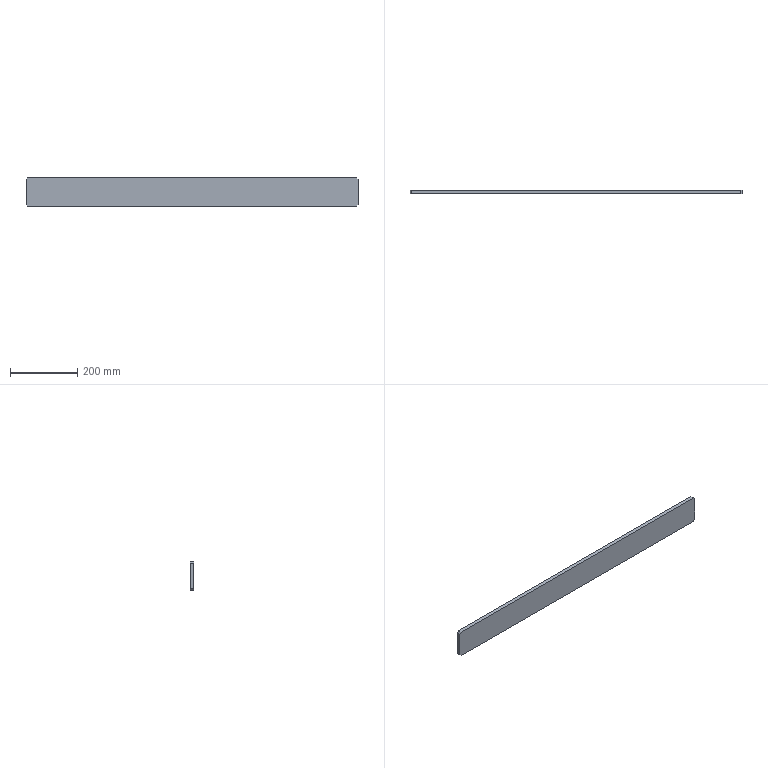Part | STEP file | Guide wheel mechanism revised.sldasm-Part-67 | 1 solid | 10 faces | box 985 x 10 x 85 mm | volume 836750 mm3 | plane 10
STEP:
#1=CARTESIAN_POINT('',(-492.5,265.,-37.5));
#2=VERTEX_POINT('',#1);
#3=CARTESIAN_POINT('',(-492.5,265.,37.5));
#4=VERTEX_POINT('',#3);
#5=CARTESIAN_POINT('',(-492.5,265.,-42.5));
#6=DIRECTION('',(0.,0.,1.));
#7=VECTOR('',#6,1000.);
#8=LINE('',#5,#7);
#9=EDGE_CURVE('',#2,#4,#8,.T.);
#10=ORIENTED_EDGE('',*,*,#9,.F.);
#11=CARTESIAN_POINT('',(-492.5,255.,-37.5));
#12=VERTEX_POINT('',#11);
#13=CARTESIAN_POINT('',(-492.5,265.,-37.5));
#14=DIRECTION('',(0.,-1.,0.));
#15=VECTOR('',#14,1000.);
#16=LINE('',#13,#15);
#17=EDGE_CURVE('',#2,#12,#16,.T.);
#18=ORIENTED_EDGE('',*,*,#17,.T.);
#19=CARTESIAN_POINT('',(-492.5,255.,37.5));
#20=VERTEX_POINT('',#19);
#21=CARTESIAN_POINT('',(-492.5,255.,-42.5));
#22=DIRECTION('',(0.,0.,1.));
#23=VECTOR('',#22,1000.);
#24=LINE('',#21,#23);
#25=EDGE_CURVE('',#12,#20,#24,.T.);
#26=ORIENTED_EDGE('',*,*,#25,.T.);
#27=CARTESIAN_POINT('',(-492.5,265.,37.5));
#28=DIRECTION('',(0.,1.,0.));
#29=VECTOR('',#28,1000.);
#30=LINE('',#27,#29);
#31=EDGE_CURVE('',#20,#4,#30,.T.);
#32=ORIENTED_EDGE('',*,*,#31,.T.);
#33=EDGE_LOOP('',(#10,#18,#26,#32));
#34=FACE_OUTER_BOUND('',#33,.T.);
#35=CARTESIAN_POINT('',(-492.5,265.,-42.5));
#36=DIRECTION('',(1.,0.,0.));
#37=DIRECTION('',(0.,0.,-1.));
#38=AXIS2_PLACEMENT_3D('',#35,#36,#37);
#39=PLANE('',#38);
#40=ADVANCED_FACE('',(#34),#39,.F.);
#41=CARTESIAN_POINT('',(-487.5,255.,42.5));
#42=VERTEX_POINT('',#41);
#43=CARTESIAN_POINT('',(487.5,255.,42.5));
#44=VERTEX_POINT('',#43);
#45=CARTESIAN_POINT('',(-492.5,255.,42.5));
#46=DIRECTION('',(1.,0.,0.));
#47=VECTOR('',#46,1000.);
#48=LINE('',#45,#47);
#49=EDGE_CURVE('',#42,#44,#48,.T.);
#50=ORIENTED_EDGE('',*,*,#49,.T.);
#51=CARTESIAN_POINT('',(487.5,265.,42.5));
#52=VERTEX_POINT('',#51);
#53=CARTESIAN_POINT('',(487.5,265.,42.5));
#54=DIRECTION('',(0.,1.,0.));
#55=VECTOR('',#54,1000.);
#56=LINE('',#53,#55);
#57=EDGE_CURVE('',#44,#52,#56,.T.);
#58=ORIENTED_EDGE('',*,*,#57,.T.);
#59=CARTESIAN_POINT('',(-487.5,265.,42.5));
#60=VERTEX_POINT('',#59);
#61=CARTESIAN_POINT('',(-492.5,265.,42.5));
#62=DIRECTION('',(1.,0.,0.));
#63=VECTOR('',#62,1000.);
#64=LINE('',#61,#63);
#65=EDGE_CURVE('',#60,#52,#64,.T.);
#66=ORIENTED_EDGE('',*,*,#65,.F.);
#67=CARTESIAN_POINT('',(-487.5,265.,42.5));
#68=DIRECTION('',(0.,-1.,0.));
#69=VECTOR('',#68,1000.);
#70=LINE('',#67,#69);
#71=EDGE_CURVE('',#60,#42,#70,.T.);
#72=ORIENTED_EDGE('',*,*,#71,.T.);
#73=EDGE_LOOP('',(#50,#58,#66,#72));
#74=FACE_OUTER_BOUND('',#73,.T.);
#75=CARTESIAN_POINT('',(-492.5,265.,42.5));
#76=DIRECTION('',(0.,0.,-1.));
#77=DIRECTION('',(-1.,0.,0.));
#78=AXIS2_PLACEMENT_3D('',#75,#76,#77);
#79=PLANE('',#78);
#80=ADVANCED_FACE('',(#74),#79,.F.);
#81=CARTESIAN_POINT('',(492.5,255.,37.5));
#82=VERTEX_POINT('',#81);
#83=CARTESIAN_POINT('',(492.5,255.,-37.5));
#84=VERTEX_POINT('',#83);
#85=CARTESIAN_POINT('',(492.5,255.,-42.5));
#86=DIRECTION('',(0.,0.,-1.));
#87=VECTOR('',#86,1000.);
#88=LINE('',#85,#87);
#89=EDGE_CURVE('',#82,#84,#88,.T.);
#90=ORIENTED_EDGE('',*,*,#89,.T.);
#91=CARTESIAN_POINT('',(492.5,265.,-37.5));
#92=VERTEX_POINT('',#91);
#93=CARTESIAN_POINT('',(492.5,265.,-37.5));
#94=DIRECTION('',(0.,1.,0.));
#95=VECTOR('',#94,1000.);
#96=LINE('',#93,#95);
#97=EDGE_CURVE('',#84,#92,#96,.T.);
#98=ORIENTED_EDGE('',*,*,#97,.T.);
#99=CARTESIAN_POINT('',(492.5,265.,37.5));
#100=VERTEX_POINT('',#99);
#101=CARTESIAN_POINT('',(492.5,265.,-42.5));
#102=DIRECTION('',(0.,0.,-1.));
#103=VECTOR('',#102,1000.);
#104=LINE('',#101,#103);
#105=EDGE_CURVE('',#100,#92,#104,.T.);
#106=ORIENTED_EDGE('',*,*,#105,.F.);
#107=CARTESIAN_POINT('',(492.5,265.,37.5));
#108=DIRECTION('',(0.,-1.,0.));
#109=VECTOR('',#108,1000.);
#110=LINE('',#107,#109);
#111=EDGE_CURVE('',#100,#82,#110,.T.);
#112=ORIENTED_EDGE('',*,*,#111,.T.);
#113=EDGE_LOOP('',(#90,#98,#106,#112));
#114=FACE_OUTER_BOUND('',#113,.T.);
#115=CARTESIAN_POINT('',(492.5,265.,-42.5));
#116=DIRECTION('',(-1.,0.,0.));
#117=DIRECTION('',(0.,0.,1.));
#118=AXIS2_PLACEMENT_3D('',#115,#116,#117);
#119=PLANE('',#118);
#120=ADVANCED_FACE('',(#114),#119,.F.);
#121=CARTESIAN_POINT('',(487.5,265.,-42.5));
#122=VERTEX_POINT('',#121);
#123=CARTESIAN_POINT('',(-487.5,265.,-42.5));
#124=VERTEX_POINT('',#123);
#125=CARTESIAN_POINT('',(-492.5,265.,-42.5));
#126=DIRECTION('',(-1.,0.,0.));
#127=VECTOR('',#126,1000.);
#128=LINE('',#125,#127);
#129=EDGE_CURVE('',#122,#124,#128,.T.);
#130=ORIENTED_EDGE('',*,*,#129,.F.);
#131=CARTESIAN_POINT('',(487.5,255.,-42.5));
#132=VERTEX_POINT('',#131);
#133=CARTESIAN_POINT('',(487.5,265.,-42.5));
#134=DIRECTION('',(0.,-1.,0.));
#135=VECTOR('',#134,1000.);
#136=LINE('',#133,#135);
#137=EDGE_CURVE('',#122,#132,#136,.T.);
#138=ORIENTED_EDGE('',*,*,#137,.T.);
#139=CARTESIAN_POINT('',(-487.5,255.,-42.5));
#140=VERTEX_POINT('',#139);
#141=CARTESIAN_POINT('',(-492.5,255.,-42.5));
#142=DIRECTION('',(-1.,0.,0.));
#143=VECTOR('',#142,1000.);
#144=LINE('',#141,#143);
#145=EDGE_CURVE('',#132,#140,#144,.T.);
#146=ORIENTED_EDGE('',*,*,#145,.T.);
#147=CARTESIAN_POINT('',(-487.5,265.,-42.5));
#148=DIRECTION('',(0.,1.,0.));
#149=VECTOR('',#148,1000.);
#150=LINE('',#147,#149);
#151=EDGE_CURVE('',#140,#124,#150,.T.);
#152=ORIENTED_EDGE('',*,*,#151,.T.);
#153=EDGE_LOOP('',(#130,#138,#146,#152));
#154=FACE_OUTER_BOUND('',#153,.T.);
#155=CARTESIAN_POINT('',(-492.5,265.,-42.5));
#156=DIRECTION('',(0.,0.,1.));
#157=DIRECTION('',(1.,0.,0.));
#158=AXIS2_PLACEMENT_3D('',#155,#156,#157);
#159=PLANE('',#158);
#160=ADVANCED_FACE('',(#154),#159,.F.);
#161=ORIENTED_EDGE('',*,*,#105,.T.);
#162=CARTESIAN_POINT('',(265.,265.,-265.));
#163=DIRECTION('',(-0.7071,0.,-0.7071));
#164=VECTOR('',#163,1000.);
#165=LINE('',#162,#164);
#166=EDGE_CURVE('',#92,#122,#165,.T.);
#167=ORIENTED_EDGE('',*,*,#166,.T.);
#168=ORIENTED_EDGE('',*,*,#129,.T.);
#169=CARTESIAN_POINT('',(-265.,265.,-265.));
#170=DIRECTION('',(-0.7071,0.,0.7071));
#171=VECTOR('',#170,1000.);
#172=LINE('',#169,#171);
#173=EDGE_CURVE('',#124,#2,#172,.T.);
#174=ORIENTED_EDGE('',*,*,#173,.T.);
#175=ORIENTED_EDGE('',*,*,#9,.T.);
#176=CARTESIAN_POINT('',(-265.,265.,265.));
#177=DIRECTION('',(0.7071,0.,0.7071));
#178=VECTOR('',#177,1000.);
#179=LINE('',#176,#178);
#180=EDGE_CURVE('',#4,#60,#179,.T.);
#181=ORIENTED_EDGE('',*,*,#180,.T.);
#182=ORIENTED_EDGE('',*,*,#65,.T.);
#183=CARTESIAN_POINT('',(265.,265.,265.));
#184=DIRECTION('',(0.7071,0.,-0.7071));
#185=VECTOR('',#184,1000.);
#186=LINE('',#183,#185);
#187=EDGE_CURVE('',#52,#100,#186,.T.);
#188=ORIENTED_EDGE('',*,*,#187,.T.);
#189=EDGE_LOOP('',(#161,#167,#168,#174,#175,#181,#182,#188));
#190=FACE_OUTER_BOUND('',#189,.T.);
#191=CARTESIAN_POINT('',(0.,265.,0.));
#192=DIRECTION('',(0.,1.,0.));
#193=DIRECTION('',(0.,0.,1.));
#194=AXIS2_PLACEMENT_3D('',#191,#192,#193);
#195=PLANE('',#194);
#196=ADVANCED_FACE('',(#190),#195,.T.);
#197=ORIENTED_EDGE('',*,*,#145,.F.);
#198=CARTESIAN_POINT('',(487.5,255.,-42.5));
#199=DIRECTION('',(0.7071,0.,0.7071));
#200=VECTOR('',#199,1000.);
#201=LINE('',#198,#200);
#202=EDGE_CURVE('',#132,#84,#201,.T.);
#203=ORIENTED_EDGE('',*,*,#202,.T.);
#204=ORIENTED_EDGE('',*,*,#89,.F.);
#205=CARTESIAN_POINT('',(492.5,255.,37.5));
#206=DIRECTION('',(-0.7071,0.,0.7071));
#207=VECTOR('',#206,1000.);
#208=LINE('',#205,#207);
#209=EDGE_CURVE('',#82,#44,#208,.T.);
#210=ORIENTED_EDGE('',*,*,#209,.T.);
#211=ORIENTED_EDGE('',*,*,#49,.F.);
#212=CARTESIAN_POINT('',(-487.5,255.,42.5));
#213=DIRECTION('',(-0.7071,0.,-0.7071));
#214=VECTOR('',#213,1000.);
#215=LINE('',#212,#214);
#216=EDGE_CURVE('',#42,#20,#215,.T.);
#217=ORIENTED_EDGE('',*,*,#216,.T.);
#218=ORIENTED_EDGE('',*,*,#25,.F.);
#219=CARTESIAN_POINT('',(-492.5,255.,-37.5));
#220=DIRECTION('',(0.7071,0.,-0.7071));
#221=VECTOR('',#220,1000.);
#222=LINE('',#219,#221);
#223=EDGE_CURVE('',#12,#140,#222,.T.);
#224=ORIENTED_EDGE('',*,*,#223,.T.);
#225=EDGE_LOOP('',(#197,#203,#204,#210,#211,#217,#218,#224));
#226=FACE_OUTER_BOUND('',#225,.T.);
#227=CARTESIAN_POINT('',(0.,255.,0.));
#228=DIRECTION('',(0.,1.,0.));
#229=DIRECTION('',(0.,0.,1.));
#230=AXIS2_PLACEMENT_3D('',#227,#228,#229);
#231=PLANE('',#230);
#232=ADVANCED_FACE('',(#226),#231,.F.);
#233=ORIENTED_EDGE('',*,*,#166,.F.);
#234=ORIENTED_EDGE('',*,*,#97,.F.);
#235=ORIENTED_EDGE('',*,*,#202,.F.);
#236=ORIENTED_EDGE('',*,*,#137,.F.);
#237=EDGE_LOOP('',(#233,#234,#235,#236));
#238=FACE_OUTER_BOUND('',#237,.T.);
#239=CARTESIAN_POINT('',(487.5,265.,-42.5));
#240=DIRECTION('',(-0.7071,0.,0.7071));
#241=DIRECTION('',(0.,-1.,0.));
#242=AXIS2_PLACEMENT_3D('',#239,#240,#241);
#243=PLANE('',#242);
#244=ADVANCED_FACE('',(#238),#243,.F.);
#245=ORIENTED_EDGE('',*,*,#187,.F.);
#246=ORIENTED_EDGE('',*,*,#57,.F.);
#247=ORIENTED_EDGE('',*,*,#209,.F.);
#248=ORIENTED_EDGE('',*,*,#111,.F.);
#249=EDGE_LOOP('',(#245,#246,#247,#248));
#250=FACE_OUTER_BOUND('',#249,.T.);
#251=CARTESIAN_POINT('',(492.5,265.,37.5));
#252=DIRECTION('',(-0.7071,0.,-0.7071));
#253=DIRECTION('',(0.,-1.,0.));
#254=AXIS2_PLACEMENT_3D('',#251,#252,#253);
#255=PLANE('',#254);
#256=ADVANCED_FACE('',(#250),#255,.F.);
#257=ORIENTED_EDGE('',*,*,#173,.F.);
#258=ORIENTED_EDGE('',*,*,#151,.F.);
#259=ORIENTED_EDGE('',*,*,#223,.F.);
#260=ORIENTED_EDGE('',*,*,#17,.F.);
#261=EDGE_LOOP('',(#257,#258,#259,#260));
#262=FACE_OUTER_BOUND('',#261,.T.);
#263=CARTESIAN_POINT('',(-492.5,265.,-37.5));
#264=DIRECTION('',(0.7071,0.,0.7071));
#265=DIRECTION('',(0.,-1.,0.));
#266=AXIS2_PLACEMENT_3D('',#263,#264,#265);
#267=PLANE('',#266);
#268=ADVANCED_FACE('',(#262),#267,.F.);
#269=ORIENTED_EDGE('',*,*,#180,.F.);
#270=ORIENTED_EDGE('',*,*,#31,.F.);
#271=ORIENTED_EDGE('',*,*,#216,.F.);
#272=ORIENTED_EDGE('',*,*,#71,.F.);
#273=EDGE_LOOP('',(#269,#270,#271,#272));
#274=FACE_OUTER_BOUND('',#273,.T.);
#275=CARTESIAN_POINT('',(-487.5,265.,42.5));
#276=DIRECTION('',(0.7071,0.,-0.7071));
#277=DIRECTION('',(0.,-1.,0.));
#278=AXIS2_PLACEMENT_3D('',#275,#276,#277);
#279=PLANE('',#278);
#280=ADVANCED_FACE('',(#274),#279,.F.);
#281=CLOSED_SHELL('',(#40,#80,#120,#160,#196,#232,#244,#256,#268,#280));
#282=MANIFOLD_SOLID_BREP('',#281);
#283=CARTESIAN_POINT('',(0.,0.,0.));
#284=DIRECTION('',(0.,0.,1.));
#285=DIRECTION('',(1.,0.,0.));
#286=AXIS2_PLACEMENT_3D('',#283,#284,#285);
#287=(LENGTH_UNIT()NAMED_UNIT(*)SI_UNIT(.MILLI.,.METRE.));
#288=UNCERTAINTY_MEASURE_WITH_UNIT(LENGTH_MEASURE(0.00001),#287,'','');
#289=(NAMED_UNIT(*)PLANE_ANGLE_UNIT()SI_UNIT($,.RADIAN.));
#290=(NAMED_UNIT(*)SI_UNIT($,.STERADIAN.)SOLID_ANGLE_UNIT());
#291=(GEOMETRIC_REPRESENTATION_CONTEXT(3)GLOBAL_UNCERTAINTY_ASSIGNED_CONTEXT((#288))GLOBAL_UNIT_ASSIGNED_CONTEXT((#287,#289,#290))REPRESENTATION_CONTEXT('',''));
#292=ADVANCED_BREP_SHAPE_REPRESENTATION('',(#282,#286),#291);